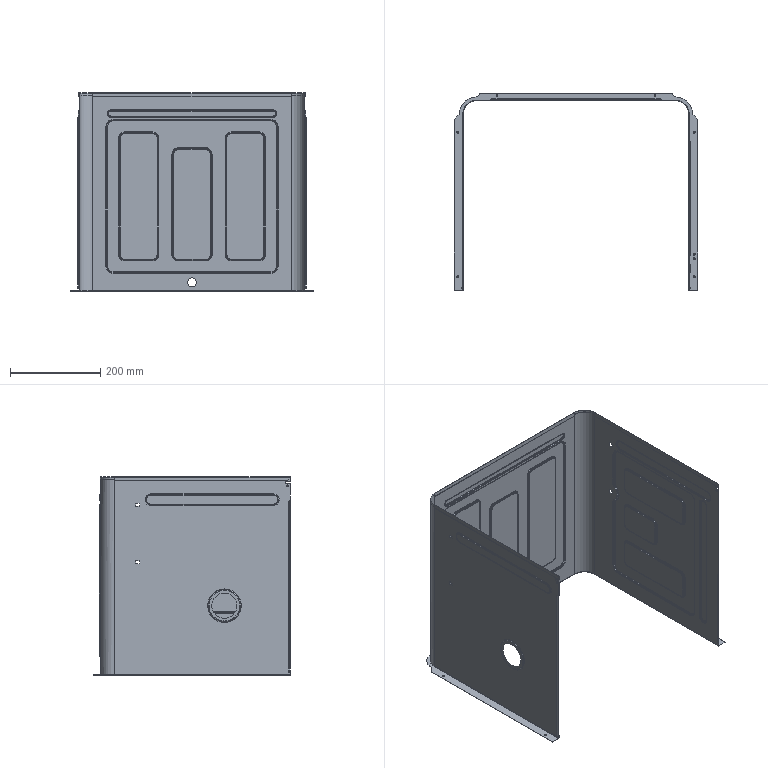Part | STEP file | ZXW722-L-01 | 1 solid | 706 faces | box 540.8 x 435.4 x 439.6 mm | volume 249280 mm3 | cylinder 253 | plane 181 | torus 170 | cone 82 | spline 20 | commonest cylinder face diameters 3 x82 3.8 x82 4 x24 2.4 x16 2 x9 6 x8